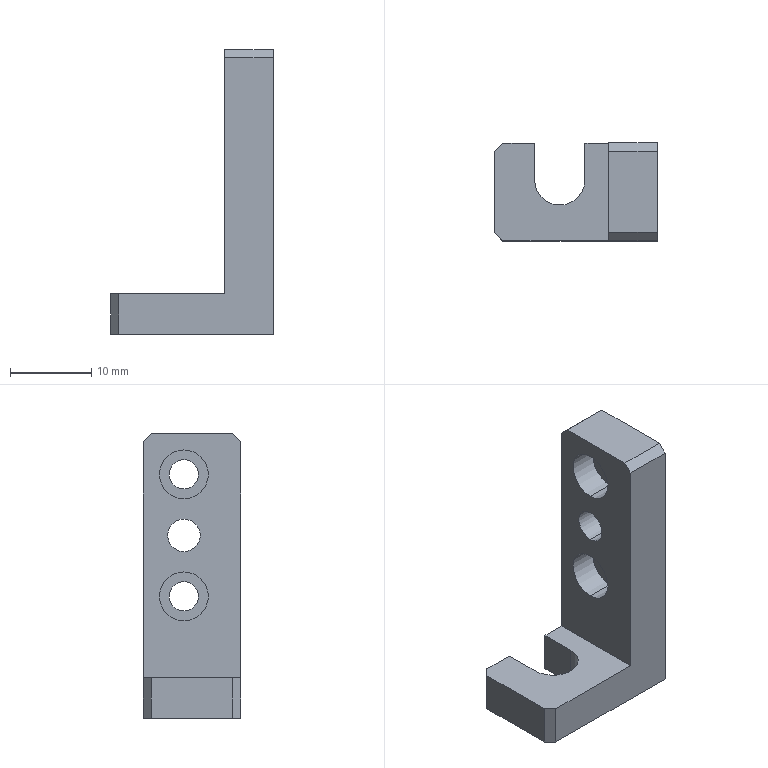Part | STEP file | 01-10 floating joint fixing plate A | 1 solid | 28 faces | box 20 x 12 x 35 mm | volume 2813 mm3 | plane 17 | cylinder 11 | commonest cylinder face diameters 3.6 x4 6 x4 4 x2 6.2 x1
STEP:
#1=CARTESIAN_POINT('',(10.,1.,20.5));
#2=VERTEX_POINT('',#1);
#3=CARTESIAN_POINT('',(10.,1.,24.5));
#4=VERTEX_POINT('',#3);
#5=CARTESIAN_POINT('',(10.,1.,22.5));
#6=DIRECTION('',(-1.,0.,0.));
#7=DIRECTION('',(0.,-1.,0.));
#8=AXIS2_PLACEMENT_3D('',#5,#6,#7);
#9=CIRCLE('',#8,2.);
#10=EDGE_CURVE('',#2,#4,#9,.T.);
#11=ORIENTED_EDGE('',*,*,#10,.F.);
#12=CARTESIAN_POINT('',(4.,1.,20.5));
#13=VERTEX_POINT('',#12);
#14=CARTESIAN_POINT('',(14.,1.,20.5));
#15=DIRECTION('',(-1.,0.,0.));
#16=VECTOR('',#15,1000.);
#17=LINE('',#14,#16);
#18=EDGE_CURVE('',#2,#13,#17,.T.);
#19=ORIENTED_EDGE('',*,*,#18,.T.);
#20=CARTESIAN_POINT('',(4.,1.,24.5));
#21=VERTEX_POINT('',#20);
#22=CARTESIAN_POINT('',(4.,1.,22.5));
#23=DIRECTION('',(-1.,0.,0.));
#24=DIRECTION('',(0.,0.,1.));
#25=AXIS2_PLACEMENT_3D('',#22,#23,#24);
#26=CIRCLE('',#25,2.);
#27=EDGE_CURVE('',#13,#21,#26,.T.);
#28=ORIENTED_EDGE('',*,*,#27,.T.);
#29=CARTESIAN_POINT('',(14.,1.,24.5));
#30=DIRECTION('',(-1.,0.,0.));
#31=VECTOR('',#30,1000.);
#32=LINE('',#29,#31);
#33=EDGE_CURVE('',#4,#21,#32,.T.);
#34=ORIENTED_EDGE('',*,*,#33,.F.);
#35=EDGE_LOOP('',(#11,#19,#28,#34));
#36=FACE_OUTER_BOUND('',#35,.T.);
#37=CARTESIAN_POINT('',(14.,1.,22.5));
#38=DIRECTION('',(-1.,0.,0.));
#39=DIRECTION('',(0.,0.,1.));
#40=AXIS2_PLACEMENT_3D('',#37,#38,#39);
#41=CYLINDRICAL_SURFACE('',#40,2.);
#42=ADVANCED_FACE('',(#36),#41,.F.);
#43=CARTESIAN_POINT('',(7.4,1.,27.));
#44=VERTEX_POINT('',#43);
#45=CARTESIAN_POINT('',(7.4,1.,33.));
#46=VERTEX_POINT('',#45);
#47=CARTESIAN_POINT('',(7.4,1.,30.));
#48=DIRECTION('',(-1.,0.,0.));
#49=DIRECTION('',(0.,0.,1.));
#50=AXIS2_PLACEMENT_3D('',#47,#48,#49);
#51=CIRCLE('',#50,3.);
#52=EDGE_CURVE('',#44,#46,#51,.T.);
#53=ORIENTED_EDGE('',*,*,#52,.F.);
#54=CARTESIAN_POINT('',(4.,1.,27.));
#55=VERTEX_POINT('',#54);
#56=CARTESIAN_POINT('',(4.,1.,27.));
#57=DIRECTION('',(-1.,0.,0.));
#58=VECTOR('',#57,1000.);
#59=LINE('',#56,#58);
#60=EDGE_CURVE('',#44,#55,#59,.T.);
#61=ORIENTED_EDGE('',*,*,#60,.T.);
#62=CARTESIAN_POINT('',(4.,1.,33.));
#63=VERTEX_POINT('',#62);
#64=CARTESIAN_POINT('',(4.,1.,30.));
#65=DIRECTION('',(-1.,0.,0.));
#66=DIRECTION('',(0.,0.,1.));
#67=AXIS2_PLACEMENT_3D('',#64,#65,#66);
#68=CIRCLE('',#67,3.);
#69=EDGE_CURVE('',#55,#63,#68,.T.);
#70=ORIENTED_EDGE('',*,*,#69,.T.);
#71=CARTESIAN_POINT('',(4.,1.,33.));
#72=DIRECTION('',(-1.,0.,0.));
#73=VECTOR('',#72,1000.);
#74=LINE('',#71,#73);
#75=EDGE_CURVE('',#46,#63,#74,.T.);
#76=ORIENTED_EDGE('',*,*,#75,.F.);
#77=EDGE_LOOP('',(#53,#61,#70,#76));
#78=FACE_OUTER_BOUND('',#77,.T.);
#79=CARTESIAN_POINT('',(4.,1.,30.));
#80=DIRECTION('',(-1.,0.,0.));
#81=DIRECTION('',(0.,0.,1.));
#82=AXIS2_PLACEMENT_3D('',#79,#80,#81);
#83=CYLINDRICAL_SURFACE('',#82,3.);
#84=ADVANCED_FACE('',(#78),#83,.F.);
#85=CARTESIAN_POINT('',(10.,1.,28.2));
#86=VERTEX_POINT('',#85);
#87=CARTESIAN_POINT('',(10.,1.,31.8));
#88=VERTEX_POINT('',#87);
#89=CARTESIAN_POINT('',(10.,1.,30.));
#90=DIRECTION('',(-1.,0.,0.));
#91=DIRECTION('',(0.,0.,1.));
#92=AXIS2_PLACEMENT_3D('',#89,#90,#91);
#93=CIRCLE('',#92,1.8);
#94=EDGE_CURVE('',#86,#88,#93,.T.);
#95=ORIENTED_EDGE('',*,*,#94,.F.);
#96=CARTESIAN_POINT('',(7.4,1.,28.2));
#97=VERTEX_POINT('',#96);
#98=CARTESIAN_POINT('',(4.,1.,28.2));
#99=DIRECTION('',(-1.,0.,0.));
#100=VECTOR('',#99,1000.);
#101=LINE('',#98,#100);
#102=EDGE_CURVE('',#86,#97,#101,.T.);
#103=ORIENTED_EDGE('',*,*,#102,.T.);
#104=CARTESIAN_POINT('',(7.4,1.,31.8));
#105=VERTEX_POINT('',#104);
#106=CARTESIAN_POINT('',(7.4,1.,30.));
#107=DIRECTION('',(-1.,0.,0.));
#108=DIRECTION('',(0.,0.,1.));
#109=AXIS2_PLACEMENT_3D('',#106,#107,#108);
#110=CIRCLE('',#109,1.8);
#111=EDGE_CURVE('',#97,#105,#110,.T.);
#112=ORIENTED_EDGE('',*,*,#111,.T.);
#113=CARTESIAN_POINT('',(4.,1.,31.8));
#114=DIRECTION('',(-1.,0.,0.));
#115=VECTOR('',#114,1000.);
#116=LINE('',#113,#115);
#117=EDGE_CURVE('',#88,#105,#116,.T.);
#118=ORIENTED_EDGE('',*,*,#117,.F.);
#119=EDGE_LOOP('',(#95,#103,#112,#118));
#120=FACE_OUTER_BOUND('',#119,.T.);
#121=CARTESIAN_POINT('',(4.,1.,30.));
#122=DIRECTION('',(-1.,0.,0.));
#123=DIRECTION('',(0.,0.,1.));
#124=AXIS2_PLACEMENT_3D('',#121,#122,#123);
#125=CYLINDRICAL_SURFACE('',#124,1.8);
#126=ADVANCED_FACE('',(#120),#125,.F.);
#127=CARTESIAN_POINT('',(7.4,1.,12.));
#128=VERTEX_POINT('',#127);
#129=CARTESIAN_POINT('',(7.4,1.,18.));
#130=VERTEX_POINT('',#129);
#131=CARTESIAN_POINT('',(7.4,1.,15.));
#132=DIRECTION('',(-1.,0.,0.));
#133=DIRECTION('',(0.,0.,1.));
#134=AXIS2_PLACEMENT_3D('',#131,#132,#133);
#135=CIRCLE('',#134,3.);
#136=EDGE_CURVE('',#128,#130,#135,.T.);
#137=ORIENTED_EDGE('',*,*,#136,.F.);
#138=CARTESIAN_POINT('',(4.,1.,12.));
#139=VERTEX_POINT('',#138);
#140=CARTESIAN_POINT('',(4.,1.,12.));
#141=DIRECTION('',(-1.,0.,0.));
#142=VECTOR('',#141,1000.);
#143=LINE('',#140,#142);
#144=EDGE_CURVE('',#128,#139,#143,.T.);
#145=ORIENTED_EDGE('',*,*,#144,.T.);
#146=CARTESIAN_POINT('',(4.,1.,18.));
#147=VERTEX_POINT('',#146);
#148=CARTESIAN_POINT('',(4.,1.,15.));
#149=DIRECTION('',(-1.,0.,0.));
#150=DIRECTION('',(0.,0.,1.));
#151=AXIS2_PLACEMENT_3D('',#148,#149,#150);
#152=CIRCLE('',#151,3.);
#153=EDGE_CURVE('',#139,#147,#152,.T.);
#154=ORIENTED_EDGE('',*,*,#153,.T.);
#155=CARTESIAN_POINT('',(4.,1.,18.));
#156=DIRECTION('',(-1.,0.,0.));
#157=VECTOR('',#156,1000.);
#158=LINE('',#155,#157);
#159=EDGE_CURVE('',#130,#147,#158,.T.);
#160=ORIENTED_EDGE('',*,*,#159,.F.);
#161=EDGE_LOOP('',(#137,#145,#154,#160));
#162=FACE_OUTER_BOUND('',#161,.T.);
#163=CARTESIAN_POINT('',(4.,1.,15.));
#164=DIRECTION('',(-1.,0.,0.));
#165=DIRECTION('',(0.,0.,1.));
#166=AXIS2_PLACEMENT_3D('',#163,#164,#165);
#167=CYLINDRICAL_SURFACE('',#166,3.);
#168=ADVANCED_FACE('',(#162),#167,.F.);
#169=CARTESIAN_POINT('',(10.,1.,13.2));
#170=VERTEX_POINT('',#169);
#171=CARTESIAN_POINT('',(10.,1.,16.8));
#172=VERTEX_POINT('',#171);
#173=CARTESIAN_POINT('',(10.,1.,15.));
#174=DIRECTION('',(-1.,0.,0.));
#175=DIRECTION('',(0.,0.,1.));
#176=AXIS2_PLACEMENT_3D('',#173,#174,#175);
#177=CIRCLE('',#176,1.8);
#178=EDGE_CURVE('',#170,#172,#177,.T.);
#179=ORIENTED_EDGE('',*,*,#178,.F.);
#180=CARTESIAN_POINT('',(7.4,1.,13.2));
#181=VERTEX_POINT('',#180);
#182=CARTESIAN_POINT('',(4.,1.,13.2));
#183=DIRECTION('',(-1.,0.,0.));
#184=VECTOR('',#183,1000.);
#185=LINE('',#182,#184);
#186=EDGE_CURVE('',#170,#181,#185,.T.);
#187=ORIENTED_EDGE('',*,*,#186,.T.);
#188=CARTESIAN_POINT('',(7.4,1.,16.8));
#189=VERTEX_POINT('',#188);
#190=CARTESIAN_POINT('',(7.4,1.,15.));
#191=DIRECTION('',(-1.,0.,0.));
#192=DIRECTION('',(0.,0.,1.));
#193=AXIS2_PLACEMENT_3D('',#190,#191,#192);
#194=CIRCLE('',#193,1.8);
#195=EDGE_CURVE('',#181,#189,#194,.T.);
#196=ORIENTED_EDGE('',*,*,#195,.T.);
#197=CARTESIAN_POINT('',(4.,1.,16.8));
#198=DIRECTION('',(-1.,0.,0.));
#199=VECTOR('',#198,1000.);
#200=LINE('',#197,#199);
#201=EDGE_CURVE('',#172,#189,#200,.T.);
#202=ORIENTED_EDGE('',*,*,#201,.F.);
#203=EDGE_LOOP('',(#179,#187,#196,#202));
#204=FACE_OUTER_BOUND('',#203,.T.);
#205=CARTESIAN_POINT('',(4.,1.,15.));
#206=DIRECTION('',(-1.,0.,0.));
#207=DIRECTION('',(0.,0.,1.));
#208=AXIS2_PLACEMENT_3D('',#205,#206,#207);
#209=CYLINDRICAL_SURFACE('',#208,1.8);
#210=ADVANCED_FACE('',(#204),#209,.F.);
#211=CARTESIAN_POINT('',(-5.1,6.,0.));
#212=VERTEX_POINT('',#211);
#213=CARTESIAN_POINT('',(-9.,6.,0.));
#214=VERTEX_POINT('',#213);
#215=CARTESIAN_POINT('',(-10.,6.,0.));
#216=DIRECTION('',(-1.,0.,0.));
#217=VECTOR('',#216,1000.);
#218=LINE('',#215,#217);
#219=EDGE_CURVE('',#212,#214,#218,.T.);
#220=ORIENTED_EDGE('',*,*,#219,.T.);
#221=CARTESIAN_POINT('',(-9.,6.,5.));
#222=VERTEX_POINT('',#221);
#223=CARTESIAN_POINT('',(-9.,6.,5.));
#224=DIRECTION('',(0.,0.,1.));
#225=VECTOR('',#224,1000.);
#226=LINE('',#223,#225);
#227=EDGE_CURVE('',#214,#222,#226,.T.);
#228=ORIENTED_EDGE('',*,*,#227,.T.);
#229=CARTESIAN_POINT('',(-5.1,6.,5.));
#230=VERTEX_POINT('',#229);
#231=CARTESIAN_POINT('',(-10.,6.,5.));
#232=DIRECTION('',(-1.,0.,0.));
#233=VECTOR('',#232,1000.);
#234=LINE('',#231,#233);
#235=EDGE_CURVE('',#230,#222,#234,.T.);
#236=ORIENTED_EDGE('',*,*,#235,.F.);
#237=CARTESIAN_POINT('',(-5.1,6.,5.));
#238=DIRECTION('',(0.,0.,-1.));
#239=VECTOR('',#238,1000.);
#240=LINE('',#237,#239);
#241=EDGE_CURVE('',#230,#212,#240,.T.);
#242=ORIENTED_EDGE('',*,*,#241,.T.);
#243=EDGE_LOOP('',(#220,#228,#236,#242));
#244=FACE_OUTER_BOUND('',#243,.T.);
#245=CARTESIAN_POINT('',(-10.,6.,5.));
#246=DIRECTION('',(0.,-1.,0.));
#247=DIRECTION('',(0.,0.,-1.));
#248=AXIS2_PLACEMENT_3D('',#245,#246,#247);
#249=PLANE('',#248);
#250=ADVANCED_FACE('',(#244),#249,.F.);
#251=CARTESIAN_POINT('',(10.,1.,22.5));
#252=DIRECTION('',(-1.,0.,0.));
#253=DIRECTION('',(0.,-1.,0.));
#254=AXIS2_PLACEMENT_3D('',#251,#252,#253);
#255=CIRCLE('',#254,2.);
#256=EDGE_CURVE('',#4,#2,#255,.T.);
#257=ORIENTED_EDGE('',*,*,#256,.T.);
#258=ORIENTED_EDGE('',*,*,#10,.T.);
#259=EDGE_LOOP('',(#257,#258));
#260=FACE_BOUND('',#259,.T.);
#261=CARTESIAN_POINT('',(10.,1.,30.));
#262=DIRECTION('',(-1.,0.,0.));
#263=DIRECTION('',(0.,0.,1.));
#264=AXIS2_PLACEMENT_3D('',#261,#262,#263);
#265=CIRCLE('',#264,1.8);
#266=EDGE_CURVE('',#88,#86,#265,.T.);
#267=ORIENTED_EDGE('',*,*,#266,.T.);
#268=ORIENTED_EDGE('',*,*,#94,.T.);
#269=EDGE_LOOP('',(#267,#268));
#270=FACE_BOUND('',#269,.T.);
#271=CARTESIAN_POINT('',(10.,1.,15.));
#272=DIRECTION('',(-1.,0.,0.));
#273=DIRECTION('',(0.,0.,1.));
#274=AXIS2_PLACEMENT_3D('',#271,#272,#273);
#275=CIRCLE('',#274,1.8);
#276=EDGE_CURVE('',#172,#170,#275,.T.);
#277=ORIENTED_EDGE('',*,*,#276,.T.);
#278=ORIENTED_EDGE('',*,*,#178,.T.);
#279=EDGE_LOOP('',(#277,#278));
#280=FACE_BOUND('',#279,.T.);
#281=CARTESIAN_POINT('',(10.,6.,34.));
#282=VERTEX_POINT('',#281);
#283=CARTESIAN_POINT('',(10.,6.,0.));
#284=VERTEX_POINT('',#283);
#285=CARTESIAN_POINT('',(10.,6.,5.));
#286=DIRECTION('',(0.,0.,-1.));
#287=VECTOR('',#286,1000.);
#288=LINE('',#285,#287);
#289=EDGE_CURVE('',#282,#284,#288,.T.);
#290=ORIENTED_EDGE('',*,*,#289,.F.);
#291=CARTESIAN_POINT('',(10.,5.,35.));
#292=VERTEX_POINT('',#291);
#293=CARTESIAN_POINT('',(10.,5.,35.));
#294=DIRECTION('',(0.,-0.7071,0.7071));
#295=VECTOR('',#294,1000.);
#296=LINE('',#293,#295);
#297=EDGE_CURVE('',#282,#292,#296,.T.);
#298=ORIENTED_EDGE('',*,*,#297,.T.);
#299=CARTESIAN_POINT('',(10.,-5.,35.));
#300=VERTEX_POINT('',#299);
#301=CARTESIAN_POINT('',(10.,-6.,35.));
#302=DIRECTION('',(0.,1.,0.));
#303=VECTOR('',#302,1000.);
#304=LINE('',#301,#303);
#305=EDGE_CURVE('',#300,#292,#304,.T.);
#306=ORIENTED_EDGE('',*,*,#305,.F.);
#307=CARTESIAN_POINT('',(10.,-6.,34.));
#308=VERTEX_POINT('',#307);
#309=CARTESIAN_POINT('',(10.,-5.,35.));
#310=DIRECTION('',(0.,-0.7071,-0.7071));
#311=VECTOR('',#310,1000.);
#312=LINE('',#309,#311);
#313=EDGE_CURVE('',#300,#308,#312,.T.);
#314=ORIENTED_EDGE('',*,*,#313,.T.);
#315=CARTESIAN_POINT('',(10.,-6.,0.));
#316=VERTEX_POINT('',#315);
#317=CARTESIAN_POINT('',(10.,-6.,5.));
#318=DIRECTION('',(0.,0.,-1.));
#319=VECTOR('',#318,1000.);
#320=LINE('',#317,#319);
#321=EDGE_CURVE('',#308,#316,#320,.T.);
#322=ORIENTED_EDGE('',*,*,#321,.T.);
#323=CARTESIAN_POINT('',(10.,6.,0.));
#324=DIRECTION('',(0.,1.,0.));
#325=VECTOR('',#324,1000.);
#326=LINE('',#323,#325);
#327=EDGE_CURVE('',#316,#284,#326,.T.);
#328=ORIENTED_EDGE('',*,*,#327,.T.);
#329=EDGE_LOOP('',(#290,#298,#306,#314,#322,#328));
#330=FACE_OUTER_BOUND('',#329,.T.);
#331=CARTESIAN_POINT('',(10.,6.,5.));
#332=DIRECTION('',(-1.,0.,0.));
#333=DIRECTION('',(0.,-1.,0.));
#334=AXIS2_PLACEMENT_3D('',#331,#332,#333);
#335=PLANE('',#334);
#336=ADVANCED_FACE('',(#260,#270,#280,#330),#335,.F.);
#337=CARTESIAN_POINT('',(4.,6.,34.));
#338=VERTEX_POINT('',#337);
#339=CARTESIAN_POINT('',(4.,6.,5.));
#340=VERTEX_POINT('',#339);
#341=CARTESIAN_POINT('',(4.,6.,35.));
#342=DIRECTION('',(0.,0.,-1.));
#343=VECTOR('',#342,1000.);
#344=LINE('',#341,#343);
#345=EDGE_CURVE('',#338,#340,#344,.T.);
#346=ORIENTED_EDGE('',*,*,#345,.F.);
#347=CARTESIAN_POINT('',(10.,6.,34.));
#348=DIRECTION('',(1.,0.,0.));
#349=VECTOR('',#348,1000.);
#350=LINE('',#347,#349);
#351=EDGE_CURVE('',#338,#282,#350,.T.);
#352=ORIENTED_EDGE('',*,*,#351,.T.);
#353=ORIENTED_EDGE('',*,*,#289,.T.);
#354=CARTESIAN_POINT('',(1.1,6.,0.));
#355=VERTEX_POINT('',#354);
#356=CARTESIAN_POINT('',(-10.,6.,0.));
#357=DIRECTION('',(-1.,0.,0.));
#358=VECTOR('',#357,1000.);
#359=LINE('',#356,#358);
#360=EDGE_CURVE('',#284,#355,#359,.T.);
#361=ORIENTED_EDGE('',*,*,#360,.T.);
#362=CARTESIAN_POINT('',(1.1,6.,5.));
#363=VERTEX_POINT('',#362);
#364=CARTESIAN_POINT('',(1.1,6.,5.));
#365=DIRECTION('',(0.,0.,1.));
#366=VECTOR('',#365,1000.);
#367=LINE('',#364,#366);
#368=EDGE_CURVE('',#355,#363,#367,.T.);
#369=ORIENTED_EDGE('',*,*,#368,.T.);
#370=CARTESIAN_POINT('',(-10.,6.,5.));
#371=DIRECTION('',(-1.,0.,0.));
#372=VECTOR('',#371,1000.);
#373=LINE('',#370,#372);
#374=EDGE_CURVE('',#340,#363,#373,.T.);
#375=ORIENTED_EDGE('',*,*,#374,.F.);
#376=EDGE_LOOP('',(#346,#352,#353,#361,#369,#375));
#377=FACE_OUTER_BOUND('',#376,.T.);
#378=CARTESIAN_POINT('',(-10.,6.,5.));
#379=DIRECTION('',(0.,-1.,0.));
#380=DIRECTION('',(0.,0.,-1.));
#381=AXIS2_PLACEMENT_3D('',#378,#379,#380);
#382=PLANE('',#381);
#383=ADVANCED_FACE('',(#377),#382,.F.);
#384=CARTESIAN_POINT('',(-10.,5.,0.));
#385=VERTEX_POINT('',#384);
#386=CARTESIAN_POINT('',(-10.,-5.,0.));
#387=VERTEX_POINT('',#386);
#388=CARTESIAN_POINT('',(-10.,6.,0.));
#389=DIRECTION('',(0.,-1.,0.));
#390=VECTOR('',#389,1000.);
#391=LINE('',#388,#390);
#392=EDGE_CURVE('',#385,#387,#391,.T.);
#393=ORIENTED_EDGE('',*,*,#392,.T.);
#394=CARTESIAN_POINT('',(-10.,-5.,5.));
#395=VERTEX_POINT('',#394);
#396=CARTESIAN_POINT('',(-10.,-5.,5.));
#397=DIRECTION('',(0.,0.,1.));
#398=VECTOR('',#397,1000.);
#399=LINE('',#396,#398);
#400=EDGE_CURVE('',#387,#395,#399,.T.);
#401=ORIENTED_EDGE('',*,*,#400,.T.);
#402=CARTESIAN_POINT('',(-10.,5.,5.));
#403=VERTEX_POINT('',#402);
#404=CARTESIAN_POINT('',(-10.,6.,5.));
#405=DIRECTION('',(0.,-1.,0.));
#406=VECTOR('',#405,1000.);
#407=LINE('',#404,#406);
#408=EDGE_CURVE('',#403,#395,#407,.T.);
#409=ORIENTED_EDGE('',*,*,#408,.F.);
#410=CARTESIAN_POINT('',(-10.,5.,5.));
#411=DIRECTION('',(0.,0.,-1.));
#412=VECTOR('',#411,1000.);
#413=LINE('',#410,#412);
#414=EDGE_CURVE('',#403,#385,#413,.T.);
#415=ORIENTED_EDGE('',*,*,#414,.T.);
#416=EDGE_LOOP('',(#393,#401,#409,#415));
#417=FACE_OUTER_BOUND('',#416,.T.);
#418=CARTESIAN_POINT('',(-10.,6.,5.));
#419=DIRECTION('',(1.,0.,0.));
#420=DIRECTION('',(0.,1.,0.));
#421=AXIS2_PLACEMENT_3D('',#418,#419,#420);
#422=PLANE('',#421);
#423=ADVANCED_FACE('',(#417),#422,.F.);
#424=CARTESIAN_POINT('',(-9.,-6.,5.));
#425=VERTEX_POINT('',#424);
#426=CARTESIAN_POINT('',(4.,-6.,5.));
#427=VERTEX_POINT('',#426);
#428=CARTESIAN_POINT('',(-10.,-6.,5.));
#429=DIRECTION('',(1.,0.,0.));
#430=VECTOR('',#429,1000.);
#431=LINE('',#428,#430);
#432=EDGE_CURVE('',#425,#427,#431,.T.);
#433=ORIENTED_EDGE('',*,*,#432,.F.);
#434=CARTESIAN_POINT('',(-9.,-6.,0.));
#435=VERTEX_POINT('',#434);
#436=CARTESIAN_POINT('',(-9.,-6.,5.));
#437=DIRECTION('',(0.,0.,-1.));
#438=VECTOR('',#437,1000.);
#439=LINE('',#436,#438);
#440=EDGE_CURVE('',#425,#435,#439,.T.);
#441=ORIENTED_EDGE('',*,*,#440,.T.);
#442=CARTESIAN_POINT('',(-10.,-6.,0.));
#443=DIRECTION('',(1.,0.,0.));
#444=VECTOR('',#443,1000.);
#445=LINE('',#442,#444);
#446=EDGE_CURVE('',#435,#316,#445,.T.);
#447=ORIENTED_EDGE('',*,*,#446,.T.);
#448=ORIENTED_EDGE('',*,*,#321,.F.);
#449=CARTESIAN_POINT('',(4.,-6.,34.));
#450=VERTEX_POINT('',#449);
#451=CARTESIAN_POINT('',(4.,-6.,34.));
#452=DIRECTION('',(-1.,0.,0.));
#453=VECTOR('',#452,1000.);
#454=LINE('',#451,#453);
#455=EDGE_CURVE('',#308,#450,#454,.T.);
#456=ORIENTED_EDGE('',*,*,#455,.T.);
#457=CARTESIAN_POINT('',(4.,-6.,35.));
#458=DIRECTION('',(0.,0.,-1.));
#459=VECTOR('',#458,1000.);
#460=LINE('',#457,#459);
#461=EDGE_CURVE('',#450,#427,#460,.T.);
#462=ORIENTED_EDGE('',*,*,#461,.T.);
#463=EDGE_LOOP('',(#433,#441,#447,#448,#456,#462));
#464=FACE_OUTER_BOUND('',#463,.T.);
#465=CARTESIAN_POINT('',(-10.,-6.,5.));
#466=DIRECTION('',(0.,1.,0.));
#467=DIRECTION('',(0.,0.,1.));
#468=AXIS2_PLACEMENT_3D('',#465,#466,#467);
#469=PLANE('',#468);
#470=ADVANCED_FACE('',(#464),#469,.F.);
#471=ORIENTED_EDGE('',*,*,#408,.T.);
#472=CARTESIAN_POINT('',(0.5,-15.5,5.));
#473=DIRECTION('',(0.7071,-0.7071,0.));
#474=VECTOR('',#473,1000.);
#475=LINE('',#472,#474);
#476=EDGE_CURVE('',#395,#425,#475,.T.);
#477=ORIENTED_EDGE('',*,*,#476,.T.);
#478=ORIENTED_EDGE('',*,*,#432,.T.);
#479=CARTESIAN_POINT('',(4.,-6.,5.));
#480=DIRECTION('',(0.,-1.,0.));
#481=VECTOR('',#480,1000.);
#482=LINE('',#479,#481);
#483=EDGE_CURVE('',#340,#427,#482,.T.);
#484=ORIENTED_EDGE('',*,*,#483,.F.);
#485=ORIENTED_EDGE('',*,*,#374,.T.);
#486=CARTESIAN_POINT('',(1.1,1.5,5.));
#487=VERTEX_POINT('',#486);
#488=CARTESIAN_POINT('',(1.1,1.5,5.));
#489=DIRECTION('',(0.,1.,0.));
#490=VECTOR('',#489,1000.);
#491=LINE('',#488,#490);
#492=EDGE_CURVE('',#487,#363,#491,.T.);
#493=ORIENTED_EDGE('',*,*,#492,.F.);
#494=CARTESIAN_POINT('',(-5.1,1.5,5.));
#495=VERTEX_POINT('',#494);
#496=CARTESIAN_POINT('',(-2.,1.5,5.));
#497=DIRECTION('',(0.,0.,1.));
#498=DIRECTION('',(1.,0.,0.));
#499=AXIS2_PLACEMENT_3D('',#496,#497,#498);
#500=CIRCLE('',#499,3.1);
#501=EDGE_CURVE('',#495,#487,#500,.T.);
#502=ORIENTED_EDGE('',*,*,#501,.F.);
#503=CARTESIAN_POINT('',(-5.1,1.5,5.));
#504=DIRECTION('',(0.,-1.,0.));
#505=VECTOR('',#504,1000.);
#506=LINE('',#503,#505);
#507=EDGE_CURVE('',#230,#495,#506,.T.);
#508=ORIENTED_EDGE('',*,*,#507,.F.);
#509=ORIENTED_EDGE('',*,*,#235,.T.);
#510=CARTESIAN_POINT('',(-5.5,9.5,5.));
#511=DIRECTION('',(-0.7071,-0.7071,0.));
#512=VECTOR('',#511,1000.);
#513=LINE('',#510,#512);
#514=EDGE_CURVE('',#222,#403,#513,.T.);
#515=ORIENTED_EDGE('',*,*,#514,.T.);
#516=EDGE_LOOP('',(#471,#477,#478,#484,#485,#493,#502,#508,#509,#515));
#517=FACE_OUTER_BOUND('',#516,.T.);
#518=CARTESIAN_POINT('',(10.,-6.,5.));
#519=DIRECTION('',(0.,0.,1.));
#520=DIRECTION('',(1.,0.,0.));
#521=AXIS2_PLACEMENT_3D('',#518,#519,#520);
#522=PLANE('',#521);
#523=ADVANCED_FACE('',(#517),#522,.T.);
#524=ORIENTED_EDGE('',*,*,#446,.F.);
#525=CARTESIAN_POINT('',(-9.,-6.,0.));
#526=DIRECTION('',(-0.7071,0.7071,0.));
#527=VECTOR('',#526,1000.);
#528=LINE('',#525,#527);
#529=EDGE_CURVE('',#435,#387,#528,.T.);
#530=ORIENTED_EDGE('',*,*,#529,.T.);
#531=ORIENTED_EDGE('',*,*,#392,.F.);
#532=CARTESIAN_POINT('',(-10.,5.,0.));
#533=DIRECTION('',(0.7071,0.7071,0.));
#534=VECTOR('',#533,1000.);
#535=LINE('',#532,#534);
#536=EDGE_CURVE('',#385,#214,#535,.T.);
#537=ORIENTED_EDGE('',*,*,#536,.T.);
#538=ORIENTED_EDGE('',*,*,#219,.F.);
#539=CARTESIAN_POINT('',(-5.1,1.5,0.));
#540=VERTEX_POINT('',#539);
#541=CARTESIAN_POINT('',(-5.1,-6.,0.));
#542=DIRECTION('',(0.,-1.,0.));
#543=VECTOR('',#542,1000.);
#544=LINE('',#541,#543);
#545=EDGE_CURVE('',#212,#540,#544,.T.);
#546=ORIENTED_EDGE('',*,*,#545,.T.);
#547=CARTESIAN_POINT('',(1.1,1.5,0.));
#548=VERTEX_POINT('',#547);
#549=CARTESIAN_POINT('',(-2.,1.5,0.));
#550=DIRECTION('',(0.,0.,1.));
#551=DIRECTION('',(1.,0.,0.));
#552=AXIS2_PLACEMENT_3D('',#549,#550,#551);
#553=CIRCLE('',#552,3.1);
#554=EDGE_CURVE('',#540,#548,#553,.T.);
#555=ORIENTED_EDGE('',*,*,#554,.T.);
#556=CARTESIAN_POINT('',(1.1,-6.,0.));
#557=DIRECTION('',(0.,1.,0.));
#558=VECTOR('',#557,1000.);
#559=LINE('',#556,#558);
#560=EDGE_CURVE('',#548,#355,#559,.T.);
#561=ORIENTED_EDGE('',*,*,#560,.T.);
#562=ORIENTED_EDGE('',*,*,#360,.F.);
#563=ORIENTED_EDGE('',*,*,#327,.F.);
#564=EDGE_LOOP('',(#524,#530,#531,#537,#538,#546,#555,#561,#562,#563));
#565=FACE_OUTER_BOUND('',#564,.T.);
#566=CARTESIAN_POINT('',(10.,-6.,0.));
#567=DIRECTION('',(0.,0.,1.));
#568=DIRECTION('',(1.,0.,0.));
#569=AXIS2_PLACEMENT_3D('',#566,#567,#568);
#570=PLANE('',#569);
#571=ADVANCED_FACE('',(#565),#570,.F.);
#572=CARTESIAN_POINT('',(4.,1.,22.5));
#573=DIRECTION('',(-1.,0.,0.));
#574=DIRECTION('',(0.,0.,1.));
#575=AXIS2_PLACEMENT_3D('',#572,#573,#574);
#576=CIRCLE('',#575,2.);
#577=EDGE_CURVE('',#21,#13,#576,.T.);
#578=ORIENTED_EDGE('',*,*,#577,.F.);
#579=ORIENTED_EDGE('',*,*,#27,.F.);
#580=EDGE_LOOP('',(#578,#579));
#581=FACE_BOUND('',#580,.T.);
#582=CARTESIAN_POINT('',(4.,1.,30.));
#583=DIRECTION('',(-1.,0.,0.));
#584=DIRECTION('',(0.,0.,1.));
#585=AXIS2_PLACEMENT_3D('',#582,#583,#584);
#586=CIRCLE('',#585,3.);
#587=EDGE_CURVE('',#63,#55,#586,.T.);
#588=ORIENTED_EDGE('',*,*,#587,.F.);
#589=ORIENTED_EDGE('',*,*,#69,.F.);
#590=EDGE_LOOP('',(#588,#589));
#591=FACE_BOUND('',#590,.T.);
#592=CARTESIAN_POINT('',(4.,1.,15.));
#593=DIRECTION('',(-1.,0.,0.));
#594=DIRECTION('',(0.,0.,1.));
#595=AXIS2_PLACEMENT_3D('',#592,#593,#594);
#596=CIRCLE('',#595,3.);
#597=EDGE_CURVE('',#147,#139,#596,.T.);
#598=ORIENTED_EDGE('',*,*,#597,.F.);
#599=ORIENTED_EDGE('',*,*,#153,.F.);
#600=EDGE_LOOP('',(#598,#599));
#601=FACE_BOUND('',#600,.T.);
#602=CARTESIAN_POINT('',(4.,5.,35.));
#603=VERTEX_POINT('',#602);
#604=CARTESIAN_POINT('',(4.,-5.,35.));
#605=VERTEX_POINT('',#604);
#606=CARTESIAN_POINT('',(4.,-6.,35.));
#607=DIRECTION('',(0.,-1.,0.));
#608=VECTOR('',#607,1000.);
#609=LINE('',#606,#608);
#610=EDGE_CURVE('',#603,#605,#609,.T.);
#611=ORIENTED_EDGE('',*,*,#610,.F.);
#612=CARTESIAN_POINT('',(4.,5.,35.));
#613=DIRECTION('',(0.,0.7071,-0.7071));
#614=VECTOR('',#613,1000.);
#615=LINE('',#612,#614);
#616=EDGE_CURVE('',#603,#338,#615,.T.);
#617=ORIENTED_EDGE('',*,*,#616,.T.);
#618=ORIENTED_EDGE('',*,*,#345,.T.);
#619=ORIENTED_EDGE('',*,*,#483,.T.);
#620=ORIENTED_EDGE('',*,*,#461,.F.);
#621=CARTESIAN_POINT('',(4.,-5.,35.));
#622=DIRECTION('',(0.,0.7071,0.7071));
#623=VECTOR('',#622,1000.);
#624=LINE('',#621,#623);
#625=EDGE_CURVE('',#450,#605,#624,.T.);
#626=ORIENTED_EDGE('',*,*,#625,.T.);
#627=EDGE_LOOP('',(#611,#617,#618,#619,#620,#626));
#628=FACE_OUTER_BOUND('',#627,.T.);
#629=CARTESIAN_POINT('',(4.,-6.,35.));
#630=DIRECTION('',(1.,0.,0.));
#631=DIRECTION('',(0.,0.,-1.));
#632=AXIS2_PLACEMENT_3D('',#629,#630,#631);
#633=PLANE('',#632);
#634=ADVANCED_FACE('',(#581,#591,#601,#628),#633,.F.);
#635=ORIENTED_EDGE('',*,*,#305,.T.);
#636=CARTESIAN_POINT('',(4.,5.,35.));
#637=DIRECTION('',(-1.,0.,0.));
#638=VECTOR('',#637,1000.);
#639=LINE('',#636,#638);
#640=EDGE_CURVE('',#292,#603,#639,.T.);
#641=ORIENTED_EDGE('',*,*,#640,.T.);
#642=ORIENTED_EDGE('',*,*,#610,.T.);
#643=CARTESIAN_POINT('',(10.,-5.,35.));
#644=DIRECTION('',(1.,0.,0.));
#645=VECTOR('',#644,1000.);
#646=LINE('',#643,#645);
#647=EDGE_CURVE('',#605,#300,#646,.T.);
#648=ORIENTED_EDGE('',*,*,#647,.T.);
#649=EDGE_LOOP('',(#635,#641,#642,#648));
#650=FACE_OUTER_BOUND('',#649,.T.);
#651=CARTESIAN_POINT('',(10.,6.,35.));
#652=DIRECTION('',(0.,0.,1.));
#653=DIRECTION('',(1.,0.,0.));
#654=AXIS2_PLACEMENT_3D('',#651,#652,#653);
#655=PLANE('',#654);
#656=ADVANCED_FACE('',(#650),#655,.T.);
#657=CARTESIAN_POINT('',(-5.1,1.5,-10.));
#658=DIRECTION('',(0.,0.,1.));
#659=VECTOR('',#658,1000.);
#660=LINE('',#657,#659);
#661=EDGE_CURVE('',#540,#495,#660,.T.);
#662=ORIENTED_EDGE('',*,*,#661,.T.);
#663=ORIENTED_EDGE('',*,*,#501,.T.);
#664=CARTESIAN_POINT('',(1.1,1.5,-10.));
#665=DIRECTION('',(0.,0.,1.));
#666=VECTOR('',#665,1000.);
#667=LINE('',#664,#666);
#668=EDGE_CURVE('',#548,#487,#667,.T.);
#669=ORIENTED_EDGE('',*,*,#668,.F.);
#670=ORIENTED_EDGE('',*,*,#554,.F.);
#671=EDGE_LOOP('',(#662,#663,#669,#670));
#672=FACE_OUTER_BOUND('',#671,.T.);
#673=CARTESIAN_POINT('',(-2.,1.5,-10.));
#674=DIRECTION('',(0.,0.,1.));
#675=DIRECTION('',(1.,0.,0.));
#676=AXIS2_PLACEMENT_3D('',#673,#674,#675);
#677=CYLINDRICAL_SURFACE('',#676,3.1);
#678=ADVANCED_FACE('',(#672),#677,.F.);
#679=ORIENTED_EDGE('',*,*,#507,.T.);
#680=ORIENTED_EDGE('',*,*,#661,.F.);
#681=ORIENTED_EDGE('',*,*,#545,.F.);
#682=ORIENTED_EDGE('',*,*,#241,.F.);
#683=EDGE_LOOP('',(#679,#680,#681,#682));
#684=FACE_OUTER_BOUND('',#683,.T.);
#685=CARTESIAN_POINT('',(-5.1,1.5,-10.));
#686=DIRECTION('',(-1.,0.,0.));
#687=DIRECTION('',(0.,0.,1.));
#688=AXIS2_PLACEMENT_3D('',#685,#686,#687);
#689=PLANE('',#688);
#690=ADVANCED_FACE('',(#684),#689,.F.);
#691=ORIENTED_EDGE('',*,*,#560,.F.);
#692=ORIENTED_EDGE('',*,*,#668,.T.);
#693=ORIENTED_EDGE('',*,*,#492,.T.);
#694=ORIENTED_EDGE('',*,*,#368,.F.);
#695=EDGE_LOOP('',(#691,#692,#693,#694));
#696=FACE_OUTER_BOUND('',#695,.T.);
#697=CARTESIAN_POINT('',(1.1,1.5,-10.));
#698=DIRECTION('',(1.,0.,0.));
#699=DIRECTION('',(0.,1.,0.));
#700=AXIS2_PLACEMENT_3D('',#697,#698,#699);
#701=PLANE('',#700);
#702=ADVANCED_FACE('',(#696),#701,.F.);
#703=ORIENTED_EDGE('',*,*,#297,.F.);
#704=ORIENTED_EDGE('',*,*,#351,.F.);
#705=ORIENTED_EDGE('',*,*,#616,.F.);
#706=ORIENTED_EDGE('',*,*,#640,.F.);
#707=EDGE_LOOP('',(#703,#704,#705,#706));
#708=FACE_OUTER_BOUND('',#707,.T.);
#709=CARTESIAN_POINT('',(10.,5.,35.));
#710=DIRECTION('',(0.,0.7071,0.7071));
#711=DIRECTION('',(0.,-0.7071,0.7071));
#712=AXIS2_PLACEMENT_3D('',#709,#710,#711);
#713=PLANE('',#712);
#714=ADVANCED_FACE('',(#708),#713,.T.);
#715=ORIENTED_EDGE('',*,*,#625,.F.);
#716=ORIENTED_EDGE('',*,*,#455,.F.);
#717=ORIENTED_EDGE('',*,*,#313,.F.);
#718=ORIENTED_EDGE('',*,*,#647,.F.);
#719=EDGE_LOOP('',(#715,#716,#717,#718));
#720=FACE_OUTER_BOUND('',#719,.T.);
#721=CARTESIAN_POINT('',(10.,-5.,35.));
#722=DIRECTION('',(0.,-0.7071,0.7071));
#723=DIRECTION('',(0.,-0.7071,-0.7071));
#724=AXIS2_PLACEMENT_3D('',#721,#722,#723);
#725=PLANE('',#724);
#726=ADVANCED_FACE('',(#720),#725,.T.);
#727=ORIENTED_EDGE('',*,*,#476,.F.);
#728=ORIENTED_EDGE('',*,*,#400,.F.);
#729=ORIENTED_EDGE('',*,*,#529,.F.);
#730=ORIENTED_EDGE('',*,*,#440,.F.);
#731=EDGE_LOOP('',(#727,#728,#729,#730));
#732=FACE_OUTER_BOUND('',#731,.T.);
#733=CARTESIAN_POINT('',(-9.,-6.,5.));
#734=DIRECTION('',(0.7071,0.7071,0.));
#735=DIRECTION('',(-0.7071,0.7071,0.));
#736=AXIS2_PLACEMENT_3D('',#733,#734,#735);
#737=PLANE('',#736);
#738=ADVANCED_FACE('',(#732),#737,.F.);
#739=ORIENTED_EDGE('',*,*,#514,.F.);
#740=ORIENTED_EDGE('',*,*,#227,.F.);
#741=ORIENTED_EDGE('',*,*,#536,.F.);
#742=ORIENTED_EDGE('',*,*,#414,.F.);
#743=EDGE_LOOP('',(#739,#740,#741,#742));
#744=FACE_OUTER_BOUND('',#743,.T.);
#745=CARTESIAN_POINT('',(-10.,5.,5.));
#746=DIRECTION('',(0.7071,-0.7071,0.));
#747=DIRECTION('',(0.7071,0.7071,0.));
#748=AXIS2_PLACEMENT_3D('',#745,#746,#747);
#749=PLANE('',#748);
#750=ADVANCED_FACE('',(#744),#749,.F.);
#751=ORIENTED_EDGE('',*,*,#186,.F.);
#752=ORIENTED_EDGE('',*,*,#276,.F.);
#753=ORIENTED_EDGE('',*,*,#201,.T.);
#754=CARTESIAN_POINT('',(7.4,1.,15.));
#755=DIRECTION('',(-1.,0.,0.));
#756=DIRECTION('',(0.,0.,1.));
#757=AXIS2_PLACEMENT_3D('',#754,#755,#756);
#758=CIRCLE('',#757,1.8);
#759=EDGE_CURVE('',#189,#181,#758,.T.);
#760=ORIENTED_EDGE('',*,*,#759,.T.);
#761=EDGE_LOOP('',(#751,#752,#753,#760));
#762=FACE_OUTER_BOUND('',#761,.T.);
#763=CARTESIAN_POINT('',(4.,1.,15.));
#764=DIRECTION('',(-1.,0.,0.));
#765=DIRECTION('',(0.,0.,1.));
#766=AXIS2_PLACEMENT_3D('',#763,#764,#765);
#767=CYLINDRICAL_SURFACE('',#766,1.8);
#768=ADVANCED_FACE('',(#762),#767,.F.);
#769=ORIENTED_EDGE('',*,*,#759,.F.);
#770=ORIENTED_EDGE('',*,*,#195,.F.);
#771=EDGE_LOOP('',(#769,#770));
#772=FACE_BOUND('',#771,.T.);
#773=CARTESIAN_POINT('',(7.4,1.,15.));
#774=DIRECTION('',(-1.,0.,0.));
#775=DIRECTION('',(0.,0.,1.));
#776=AXIS2_PLACEMENT_3D('',#773,#774,#775);
#777=CIRCLE('',#776,3.);
#778=EDGE_CURVE('',#130,#128,#777,.T.);
#779=ORIENTED_EDGE('',*,*,#778,.T.);
#780=ORIENTED_EDGE('',*,*,#136,.T.);
#781=EDGE_LOOP('',(#779,#780));
#782=FACE_OUTER_BOUND('',#781,.T.);
#783=CARTESIAN_POINT('',(7.4,2.8,15.));
#784=DIRECTION('',(1.,0.,0.));
#785=DIRECTION('',(0.,0.,-1.));
#786=AXIS2_PLACEMENT_3D('',#783,#784,#785);
#787=PLANE('',#786);
#788=ADVANCED_FACE('',(#772,#782),#787,.F.);
#789=ORIENTED_EDGE('',*,*,#144,.F.);
#790=ORIENTED_EDGE('',*,*,#778,.F.);
#791=ORIENTED_EDGE('',*,*,#159,.T.);
#792=ORIENTED_EDGE('',*,*,#597,.T.);
#793=EDGE_LOOP('',(#789,#790,#791,#792));
#794=FACE_OUTER_BOUND('',#793,.T.);
#795=CARTESIAN_POINT('',(4.,1.,15.));
#796=DIRECTION('',(-1.,0.,0.));
#797=DIRECTION('',(0.,0.,1.));
#798=AXIS2_PLACEMENT_3D('',#795,#796,#797);
#799=CYLINDRICAL_SURFACE('',#798,3.);
#800=ADVANCED_FACE('',(#794),#799,.F.);
#801=ORIENTED_EDGE('',*,*,#102,.F.);
#802=ORIENTED_EDGE('',*,*,#266,.F.);
#803=ORIENTED_EDGE('',*,*,#117,.T.);
#804=CARTESIAN_POINT('',(7.4,1.,30.));
#805=DIRECTION('',(-1.,0.,0.));
#806=DIRECTION('',(0.,0.,1.));
#807=AXIS2_PLACEMENT_3D('',#804,#805,#806);
#808=CIRCLE('',#807,1.8);
#809=EDGE_CURVE('',#105,#97,#808,.T.);
#810=ORIENTED_EDGE('',*,*,#809,.T.);
#811=EDGE_LOOP('',(#801,#802,#803,#810));
#812=FACE_OUTER_BOUND('',#811,.T.);
#813=CARTESIAN_POINT('',(4.,1.,30.));
#814=DIRECTION('',(-1.,0.,0.));
#815=DIRECTION('',(0.,0.,1.));
#816=AXIS2_PLACEMENT_3D('',#813,#814,#815);
#817=CYLINDRICAL_SURFACE('',#816,1.8);
#818=ADVANCED_FACE('',(#812),#817,.F.);
#819=ORIENTED_EDGE('',*,*,#809,.F.);
#820=ORIENTED_EDGE('',*,*,#111,.F.);
#821=EDGE_LOOP('',(#819,#820));
#822=FACE_BOUND('',#821,.T.);
#823=CARTESIAN_POINT('',(7.4,1.,30.));
#824=DIRECTION('',(-1.,0.,0.));
#825=DIRECTION('',(0.,0.,1.));
#826=AXIS2_PLACEMENT_3D('',#823,#824,#825);
#827=CIRCLE('',#826,3.);
#828=EDGE_CURVE('',#46,#44,#827,.T.);
#829=ORIENTED_EDGE('',*,*,#828,.T.);
#830=ORIENTED_EDGE('',*,*,#52,.T.);
#831=EDGE_LOOP('',(#829,#830));
#832=FACE_OUTER_BOUND('',#831,.T.);
#833=CARTESIAN_POINT('',(7.4,2.8,30.));
#834=DIRECTION('',(1.,0.,0.));
#835=DIRECTION('',(0.,0.,-1.));
#836=AXIS2_PLACEMENT_3D('',#833,#834,#835);
#837=PLANE('',#836);
#838=ADVANCED_FACE('',(#822,#832),#837,.F.);
#839=ORIENTED_EDGE('',*,*,#60,.F.);
#840=ORIENTED_EDGE('',*,*,#828,.F.);
#841=ORIENTED_EDGE('',*,*,#75,.T.);
#842=ORIENTED_EDGE('',*,*,#587,.T.);
#843=EDGE_LOOP('',(#839,#840,#841,#842));
#844=FACE_OUTER_BOUND('',#843,.T.);
#845=CARTESIAN_POINT('',(4.,1.,30.));
#846=DIRECTION('',(-1.,0.,0.));
#847=DIRECTION('',(0.,0.,1.));
#848=AXIS2_PLACEMENT_3D('',#845,#846,#847);
#849=CYLINDRICAL_SURFACE('',#848,3.);
#850=ADVANCED_FACE('',(#844),#849,.F.);
#851=ORIENTED_EDGE('',*,*,#18,.F.);
#852=ORIENTED_EDGE('',*,*,#256,.F.);
#853=ORIENTED_EDGE('',*,*,#33,.T.);
#854=ORIENTED_EDGE('',*,*,#577,.T.);
#855=EDGE_LOOP('',(#851,#852,#853,#854));
#856=FACE_OUTER_BOUND('',#855,.T.);
#857=CARTESIAN_POINT('',(14.,1.,22.5));
#858=DIRECTION('',(-1.,0.,0.));
#859=DIRECTION('',(0.,0.,1.));
#860=AXIS2_PLACEMENT_3D('',#857,#858,#859);
#861=CYLINDRICAL_SURFACE('',#860,2.);
#862=ADVANCED_FACE('',(#856),#861,.F.);
#863=CLOSED_SHELL('',(#42,#84,#126,#168,#210,#250,#336,#383,#423,#470,#523,#571,#634,#656,#678,#690,#702,#714,#726,#738,#750,#768,#788,#800,#818,#838,#850,#862));
#864=MANIFOLD_SOLID_BREP('',#863);
#865=CARTESIAN_POINT('',(0.,0.,0.));
#866=DIRECTION('',(0.,0.,1.));
#867=DIRECTION('',(1.,0.,0.));
#868=AXIS2_PLACEMENT_3D('',#865,#866,#867);
#869=(LENGTH_UNIT()NAMED_UNIT(*)SI_UNIT(.MILLI.,.METRE.));
#870=UNCERTAINTY_MEASURE_WITH_UNIT(LENGTH_MEASURE(0.00001),#869,'','');
#871=(NAMED_UNIT(*)PLANE_ANGLE_UNIT()SI_UNIT($,.RADIAN.));
#872=(NAMED_UNIT(*)SI_UNIT($,.STERADIAN.)SOLID_ANGLE_UNIT());
#873=(GEOMETRIC_REPRESENTATION_CONTEXT(3)GLOBAL_UNCERTAINTY_ASSIGNED_CONTEXT((#870))GLOBAL_UNIT_ASSIGNED_CONTEXT((#869,#871,#872))REPRESENTATION_CONTEXT('',''));
#874=ADVANCED_BREP_SHAPE_REPRESENTATION('',(#864,#868),#873);